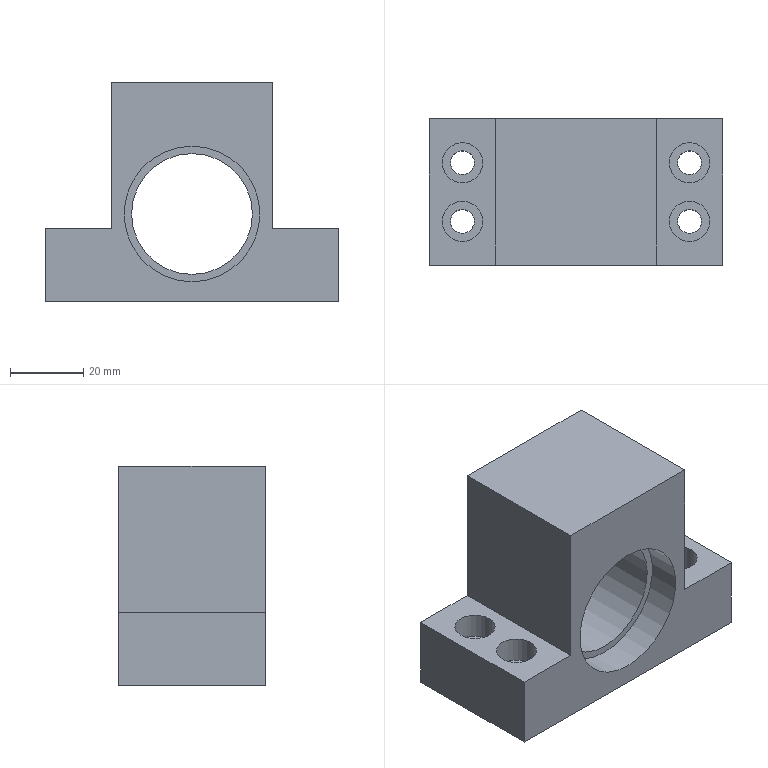Part | NX | features CBORE_HOLE 5, DATUM_CSYS 5, SKETCH 4, EXTRUDE 2, HOLE PACKAGE 2 | 1 solid | 25 faces | box 80 x 40 x 60 mm | volume 93822 mm3 | plane 15 | cylinder 10 | commonest cylinder face diameters 6.5 x4 11 x4 33 x1 37 x1
STEP:
#1=CARTESIAN_POINT('',(22.,20.,30.));
#2=VERTEX_POINT('',#1);
#3=CARTESIAN_POINT('',(22.,-20.,30.));
#4=VERTEX_POINT('',#3);
#5=CARTESIAN_POINT('',(22.,24.,30.));
#6=DIRECTION('',(0.,-1.,0.));
#7=VECTOR('',#6,1000.);
#8=LINE('',#5,#7);
#9=EDGE_CURVE('',#2,#4,#8,.T.);
#10=ORIENTED_EDGE('',*,*,#9,.F.);
#11=CARTESIAN_POINT('',(-22.,20.,30.));
#12=VERTEX_POINT('',#11);
#13=CARTESIAN_POINT('',(40.,20.,30.));
#14=DIRECTION('',(-1.,0.,0.));
#15=VECTOR('',#14,1000.);
#16=LINE('',#13,#15);
#17=EDGE_CURVE('',#2,#12,#16,.T.);
#18=ORIENTED_EDGE('',*,*,#17,.T.);
#19=CARTESIAN_POINT('',(-22.,-20.,30.));
#20=VERTEX_POINT('',#19);
#21=CARTESIAN_POINT('',(-22.,24.,30.));
#22=DIRECTION('',(0.,-1.,0.));
#23=VECTOR('',#22,1000.);
#24=LINE('',#21,#23);
#25=EDGE_CURVE('',#12,#20,#24,.T.);
#26=ORIENTED_EDGE('',*,*,#25,.T.);
#27=CARTESIAN_POINT('',(40.,-20.,30.));
#28=DIRECTION('',(-1.,0.,0.));
#29=VECTOR('',#28,1000.);
#30=LINE('',#27,#29);
#31=EDGE_CURVE('',#4,#20,#30,.T.);
#32=ORIENTED_EDGE('',*,*,#31,.F.);
#33=EDGE_LOOP('',(#10,#18,#26,#32));
#34=FACE_BOUND('',#33,.T.);
#35=CARTESIAN_POINT('',(40.,-20.,30.));
#36=DIRECTION('',(0.,0.,-1.));
#37=DIRECTION('',(-1.,0.,0.));
#38=AXIS2_PLACEMENT_3D('',#35,#36,#37);
#39=PLANE('',#38);
#40=ADVANCED_FACE('',(#34),#39,.F.);
#41=CARTESIAN_POINT('',(-40.,20.,-10.));
#42=VERTEX_POINT('',#41);
#43=CARTESIAN_POINT('',(-40.,-20.,-10.));
#44=VERTEX_POINT('',#43);
#45=CARTESIAN_POINT('',(-40.,24.,-10.));
#46=DIRECTION('',(0.,-1.,0.));
#47=VECTOR('',#46,1000.);
#48=LINE('',#45,#47);
#49=EDGE_CURVE('',#42,#44,#48,.T.);
#50=ORIENTED_EDGE('',*,*,#49,.F.);
#51=CARTESIAN_POINT('',(-40.,20.,-30.));
#52=VERTEX_POINT('',#51);
#53=CARTESIAN_POINT('',(-40.,20.,30.));
#54=DIRECTION('',(0.,0.,-1.));
#55=VECTOR('',#54,1000.);
#56=LINE('',#53,#55);
#57=EDGE_CURVE('',#42,#52,#56,.T.);
#58=ORIENTED_EDGE('',*,*,#57,.T.);
#59=CARTESIAN_POINT('',(-40.,-20.,-30.));
#60=VERTEX_POINT('',#59);
#61=CARTESIAN_POINT('',(-40.,-20.,-30.));
#62=DIRECTION('',(0.,1.,0.));
#63=VECTOR('',#62,1000.);
#64=LINE('',#61,#63);
#65=EDGE_CURVE('',#60,#52,#64,.T.);
#66=ORIENTED_EDGE('',*,*,#65,.F.);
#67=CARTESIAN_POINT('',(-40.,-20.,30.));
#68=DIRECTION('',(0.,0.,-1.));
#69=VECTOR('',#68,1000.);
#70=LINE('',#67,#69);
#71=EDGE_CURVE('',#44,#60,#70,.T.);
#72=ORIENTED_EDGE('',*,*,#71,.F.);
#73=EDGE_LOOP('',(#50,#58,#66,#72));
#74=FACE_BOUND('',#73,.T.);
#75=CARTESIAN_POINT('',(-40.,-20.,30.));
#76=DIRECTION('',(1.,0.,0.));
#77=DIRECTION('',(0.,0.,-1.));
#78=AXIS2_PLACEMENT_3D('',#75,#76,#77);
#79=PLANE('',#78);
#80=ADVANCED_FACE('',(#74),#79,.F.);
#81=CARTESIAN_POINT('',(34.25,8.,-30.));
#82=VERTEX_POINT('',#81);
#83=CARTESIAN_POINT('',(31.,8.,-30.));
#84=DIRECTION('',(0.,0.,1.));
#85=DIRECTION('',(1.,0.,0.));
#86=AXIS2_PLACEMENT_3D('',#83,#84,#85);
#87=CIRCLE('',#86,3.25);
#88=EDGE_CURVE('',#82,#82,#87,.T.);
#89=ORIENTED_EDGE('',*,*,#88,.T.);
#90=EDGE_LOOP('',(#89));
#91=FACE_BOUND('',#90,.T.);
#92=CARTESIAN_POINT('',(34.25,-8.,-30.));
#93=VERTEX_POINT('',#92);
#94=CARTESIAN_POINT('',(31.,-8.,-30.));
#95=DIRECTION('',(0.,0.,1.));
#96=DIRECTION('',(1.,0.,0.));
#97=AXIS2_PLACEMENT_3D('',#94,#95,#96);
#98=CIRCLE('',#97,3.25);
#99=EDGE_CURVE('',#93,#93,#98,.T.);
#100=ORIENTED_EDGE('',*,*,#99,.T.);
#101=EDGE_LOOP('',(#100));
#102=FACE_BOUND('',#101,.T.);
#103=CARTESIAN_POINT('',(-27.75,8.,-30.));
#104=VERTEX_POINT('',#103);
#105=CARTESIAN_POINT('',(-31.,8.,-30.));
#106=DIRECTION('',(0.,0.,1.));
#107=DIRECTION('',(1.,0.,0.));
#108=AXIS2_PLACEMENT_3D('',#105,#106,#107);
#109=CIRCLE('',#108,3.25);
#110=EDGE_CURVE('',#104,#104,#109,.T.);
#111=ORIENTED_EDGE('',*,*,#110,.T.);
#112=EDGE_LOOP('',(#111));
#113=FACE_BOUND('',#112,.T.);
#114=CARTESIAN_POINT('',(-27.75,-8.,-30.));
#115=VERTEX_POINT('',#114);
#116=CARTESIAN_POINT('',(-31.,-8.,-30.));
#117=DIRECTION('',(0.,0.,1.));
#118=DIRECTION('',(1.,0.,0.));
#119=AXIS2_PLACEMENT_3D('',#116,#117,#118);
#120=CIRCLE('',#119,3.25);
#121=EDGE_CURVE('',#115,#115,#120,.T.);
#122=ORIENTED_EDGE('',*,*,#121,.T.);
#123=EDGE_LOOP('',(#122));
#124=FACE_BOUND('',#123,.T.);
#125=CARTESIAN_POINT('',(40.,20.,-30.));
#126=VERTEX_POINT('',#125);
#127=CARTESIAN_POINT('',(-40.,20.,-30.));
#128=DIRECTION('',(1.,0.,0.));
#129=VECTOR('',#128,1000.);
#130=LINE('',#127,#129);
#131=EDGE_CURVE('',#52,#126,#130,.T.);
#132=ORIENTED_EDGE('',*,*,#131,.T.);
#133=CARTESIAN_POINT('',(40.,-20.,-30.));
#134=VERTEX_POINT('',#133);
#135=CARTESIAN_POINT('',(40.,-20.,-30.));
#136=DIRECTION('',(0.,1.,0.));
#137=VECTOR('',#136,1000.);
#138=LINE('',#135,#137);
#139=EDGE_CURVE('',#134,#126,#138,.T.);
#140=ORIENTED_EDGE('',*,*,#139,.F.);
#141=CARTESIAN_POINT('',(-40.,-20.,-30.));
#142=DIRECTION('',(1.,0.,0.));
#143=VECTOR('',#142,1000.);
#144=LINE('',#141,#143);
#145=EDGE_CURVE('',#60,#134,#144,.T.);
#146=ORIENTED_EDGE('',*,*,#145,.F.);
#147=ORIENTED_EDGE('',*,*,#65,.T.);
#148=EDGE_LOOP('',(#132,#140,#146,#147));
#149=FACE_BOUND('',#148,.T.);
#150=CARTESIAN_POINT('',(-40.,-20.,-30.));
#151=DIRECTION('',(0.,0.,1.));
#152=DIRECTION('',(1.,0.,0.));
#153=AXIS2_PLACEMENT_3D('',#150,#151,#152);
#154=PLANE('',#153);
#155=ADVANCED_FACE('',(#91,#102,#113,#124,#149),#154,.F.);
#156=CARTESIAN_POINT('',(40.,20.,-10.));
#157=VERTEX_POINT('',#156);
#158=CARTESIAN_POINT('',(40.,20.,-30.));
#159=DIRECTION('',(0.,0.,1.));
#160=VECTOR('',#159,1000.);
#161=LINE('',#158,#160);
#162=EDGE_CURVE('',#126,#157,#161,.T.);
#163=ORIENTED_EDGE('',*,*,#162,.T.);
#164=CARTESIAN_POINT('',(40.,-20.,-10.));
#165=VERTEX_POINT('',#164);
#166=CARTESIAN_POINT('',(40.,24.,-10.));
#167=DIRECTION('',(0.,-1.,0.));
#168=VECTOR('',#167,1000.);
#169=LINE('',#166,#168);
#170=EDGE_CURVE('',#157,#165,#169,.T.);
#171=ORIENTED_EDGE('',*,*,#170,.T.);
#172=CARTESIAN_POINT('',(40.,-20.,-30.));
#173=DIRECTION('',(0.,0.,1.));
#174=VECTOR('',#173,1000.);
#175=LINE('',#172,#174);
#176=EDGE_CURVE('',#134,#165,#175,.T.);
#177=ORIENTED_EDGE('',*,*,#176,.F.);
#178=ORIENTED_EDGE('',*,*,#139,.T.);
#179=EDGE_LOOP('',(#163,#171,#177,#178));
#180=FACE_BOUND('',#179,.T.);
#181=CARTESIAN_POINT('',(40.,-20.,-30.));
#182=DIRECTION('',(-1.,0.,0.));
#183=DIRECTION('',(0.,0.,1.));
#184=AXIS2_PLACEMENT_3D('',#181,#182,#183);
#185=PLANE('',#184);
#186=ADVANCED_FACE('',(#180),#185,.F.);
#187=CARTESIAN_POINT('',(22.,-20.,-10.));
#188=VERTEX_POINT('',#187);
#189=CARTESIAN_POINT('',(22.,-20.,30.));
#190=DIRECTION('',(0.,0.,-1.));
#191=VECTOR('',#190,1000.);
#192=LINE('',#189,#191);
#193=EDGE_CURVE('',#4,#188,#192,.T.);
#194=ORIENTED_EDGE('',*,*,#193,.F.);
#195=ORIENTED_EDGE('',*,*,#31,.T.);
#196=CARTESIAN_POINT('',(-22.,-20.,-10.));
#197=VERTEX_POINT('',#196);
#198=CARTESIAN_POINT('',(-22.,-20.,-10.));
#199=DIRECTION('',(0.,0.,1.));
#200=VECTOR('',#199,1000.);
#201=LINE('',#198,#200);
#202=EDGE_CURVE('',#197,#20,#201,.T.);
#203=ORIENTED_EDGE('',*,*,#202,.F.);
#204=CARTESIAN_POINT('',(-40.,-20.,-10.));
#205=DIRECTION('',(1.,0.,0.));
#206=VECTOR('',#205,1000.);
#207=LINE('',#204,#206);
#208=EDGE_CURVE('',#44,#197,#207,.T.);
#209=ORIENTED_EDGE('',*,*,#208,.F.);
#210=ORIENTED_EDGE('',*,*,#71,.T.);
#211=ORIENTED_EDGE('',*,*,#145,.T.);
#212=ORIENTED_EDGE('',*,*,#176,.T.);
#213=CARTESIAN_POINT('',(22.,-20.,-10.));
#214=DIRECTION('',(1.,0.,0.));
#215=VECTOR('',#214,1000.);
#216=LINE('',#213,#215);
#217=EDGE_CURVE('',#188,#165,#216,.T.);
#218=ORIENTED_EDGE('',*,*,#217,.F.);
#219=EDGE_LOOP('',(#194,#195,#203,#209,#210,#211,#212,#218));
#220=FACE_BOUND('',#219,.T.);
#221=CARTESIAN_POINT('',(0.,-20.,12.5));
#222=VERTEX_POINT('',#221);
#223=CARTESIAN_POINT('',(0.,-20.,-6.));
#224=DIRECTION('',(0.,1.,0.));
#225=DIRECTION('',(0.,0.,1.));
#226=AXIS2_PLACEMENT_3D('',#223,#224,#225);
#227=CIRCLE('',#226,18.5);
#228=EDGE_CURVE('',#222,#222,#227,.T.);
#229=ORIENTED_EDGE('',*,*,#228,.T.);
#230=EDGE_LOOP('',(#229));
#231=FACE_BOUND('',#230,.T.);
#232=CARTESIAN_POINT('',(0.,-20.,0.));
#233=DIRECTION('',(0.,-1.,0.));
#234=DIRECTION('',(0.,0.,-1.));
#235=AXIS2_PLACEMENT_3D('',#232,#233,#234);
#236=PLANE('',#235);
#237=ADVANCED_FACE('',(#220,#231),#236,.T.);
#238=CARTESIAN_POINT('',(0.,20.,-22.5));
#239=VERTEX_POINT('',#238);
#240=CARTESIAN_POINT('',(0.,20.,-6.));
#241=DIRECTION('',(0.,-1.,0.));
#242=DIRECTION('',(0.,0.,-1.));
#243=AXIS2_PLACEMENT_3D('',#240,#241,#242);
#244=CIRCLE('',#243,16.5);
#245=EDGE_CURVE('',#239,#239,#244,.T.);
#246=ORIENTED_EDGE('',*,*,#245,.T.);
#247=EDGE_LOOP('',(#246));
#248=FACE_BOUND('',#247,.T.);
#249=ORIENTED_EDGE('',*,*,#17,.F.);
#250=CARTESIAN_POINT('',(22.,20.,-10.));
#251=VERTEX_POINT('',#250);
#252=CARTESIAN_POINT('',(22.,20.,0.));
#253=DIRECTION('',(0.,0.,-1.));
#254=VECTOR('',#253,1000.);
#255=LINE('',#252,#254);
#256=EDGE_CURVE('',#2,#251,#255,.T.);
#257=ORIENTED_EDGE('',*,*,#256,.T.);
#258=CARTESIAN_POINT('',(0.,20.,-10.));
#259=DIRECTION('',(1.,0.,0.));
#260=VECTOR('',#259,1000.);
#261=LINE('',#258,#260);
#262=EDGE_CURVE('',#251,#157,#261,.T.);
#263=ORIENTED_EDGE('',*,*,#262,.T.);
#264=ORIENTED_EDGE('',*,*,#162,.F.);
#265=ORIENTED_EDGE('',*,*,#131,.F.);
#266=ORIENTED_EDGE('',*,*,#57,.F.);
#267=CARTESIAN_POINT('',(-22.,20.,-10.));
#268=VERTEX_POINT('',#267);
#269=CARTESIAN_POINT('',(0.,20.,-10.));
#270=DIRECTION('',(1.,0.,0.));
#271=VECTOR('',#270,1000.);
#272=LINE('',#269,#271);
#273=EDGE_CURVE('',#42,#268,#272,.T.);
#274=ORIENTED_EDGE('',*,*,#273,.T.);
#275=CARTESIAN_POINT('',(-22.,20.,0.));
#276=DIRECTION('',(0.,0.,1.));
#277=VECTOR('',#276,1000.);
#278=LINE('',#275,#277);
#279=EDGE_CURVE('',#268,#12,#278,.T.);
#280=ORIENTED_EDGE('',*,*,#279,.T.);
#281=EDGE_LOOP('',(#249,#257,#263,#264,#265,#266,#274,#280));
#282=FACE_BOUND('',#281,.T.);
#283=CARTESIAN_POINT('',(0.,20.,0.));
#284=DIRECTION('',(0.,-1.,0.));
#285=DIRECTION('',(0.,0.,-1.));
#286=AXIS2_PLACEMENT_3D('',#283,#284,#285);
#287=PLANE('',#286);
#288=ADVANCED_FACE('',(#248,#282),#287,.F.);
#289=CARTESIAN_POINT('',(0.,-11.,10.5));
#290=VERTEX_POINT('',#289);
#291=CARTESIAN_POINT('',(0.,-11.,-6.));
#292=DIRECTION('',(0.,1.,0.));
#293=DIRECTION('',(0.,0.,1.));
#294=AXIS2_PLACEMENT_3D('',#291,#292,#293);
#295=CIRCLE('',#294,16.5);
#296=EDGE_CURVE('',#290,#290,#295,.F.);
#297=ORIENTED_EDGE('',*,*,#296,.T.);
#298=EDGE_LOOP('',(#297));
#299=FACE_BOUND('',#298,.T.);
#300=ORIENTED_EDGE('',*,*,#245,.F.);
#301=EDGE_LOOP('',(#300));
#302=FACE_BOUND('',#301,.T.);
#303=CARTESIAN_POINT('',(0.,58.932,-6.));
#304=DIRECTION('',(0.,1.,0.));
#305=DIRECTION('',(0.,0.,1.));
#306=AXIS2_PLACEMENT_3D('',#303,#304,#305);
#307=CYLINDRICAL_SURFACE('',#306,16.5);
#308=ADVANCED_FACE('',(#299,#302),#307,.F.);
#309=ORIENTED_EDGE('',*,*,#296,.F.);
#310=EDGE_LOOP('',(#309));
#311=FACE_BOUND('',#310,.T.);
#312=CARTESIAN_POINT('',(0.,-11.,12.5));
#313=VERTEX_POINT('',#312);
#314=CARTESIAN_POINT('',(0.,-11.,-6.));
#315=DIRECTION('',(0.,1.,0.));
#316=DIRECTION('',(0.,0.,1.));
#317=AXIS2_PLACEMENT_3D('',#314,#315,#316);
#318=CIRCLE('',#317,18.5);
#319=EDGE_CURVE('',#313,#313,#318,.F.);
#320=ORIENTED_EDGE('',*,*,#319,.T.);
#321=EDGE_LOOP('',(#320));
#322=FACE_BOUND('',#321,.T.);
#323=CARTESIAN_POINT('',(0.,-11.,-6.));
#324=DIRECTION('',(0.,1.,0.));
#325=DIRECTION('',(0.,0.,1.));
#326=AXIS2_PLACEMENT_3D('',#323,#324,#325);
#327=PLANE('',#326);
#328=ADVANCED_FACE('',(#311,#322),#327,.F.);
#329=ORIENTED_EDGE('',*,*,#319,.F.);
#330=EDGE_LOOP('',(#329));
#331=FACE_BOUND('',#330,.T.);
#332=ORIENTED_EDGE('',*,*,#228,.F.);
#333=EDGE_LOOP('',(#332));
#334=FACE_BOUND('',#333,.T.);
#335=CARTESIAN_POINT('',(0.,-20.,-6.));
#336=DIRECTION('',(0.,1.,0.));
#337=DIRECTION('',(0.,0.,1.));
#338=AXIS2_PLACEMENT_3D('',#335,#336,#337);
#339=CYLINDRICAL_SURFACE('',#338,18.5);
#340=ADVANCED_FACE('',(#331,#334),#339,.F.);
#341=CARTESIAN_POINT('',(-36.5,8.,-10.));
#342=VERTEX_POINT('',#341);
#343=CARTESIAN_POINT('',(-31.,8.,-10.));
#344=DIRECTION('',(0.,0.,-1.));
#345=DIRECTION('',(-1.,0.,0.));
#346=AXIS2_PLACEMENT_3D('',#343,#344,#345);
#347=CIRCLE('',#346,5.5);
#348=EDGE_CURVE('',#342,#342,#347,.T.);
#349=ORIENTED_EDGE('',*,*,#348,.T.);
#350=EDGE_LOOP('',(#349));
#351=FACE_BOUND('',#350,.T.);
#352=CARTESIAN_POINT('',(-36.5,-8.,-10.));
#353=VERTEX_POINT('',#352);
#354=CARTESIAN_POINT('',(-31.,-8.,-10.));
#355=DIRECTION('',(0.,0.,-1.));
#356=DIRECTION('',(-1.,0.,0.));
#357=AXIS2_PLACEMENT_3D('',#354,#355,#356);
#358=CIRCLE('',#357,5.5);
#359=EDGE_CURVE('',#353,#353,#358,.T.);
#360=ORIENTED_EDGE('',*,*,#359,.T.);
#361=EDGE_LOOP('',(#360));
#362=FACE_BOUND('',#361,.T.);
#363=ORIENTED_EDGE('',*,*,#49,.T.);
#364=ORIENTED_EDGE('',*,*,#208,.T.);
#365=CARTESIAN_POINT('',(-22.,24.,-10.));
#366=DIRECTION('',(0.,-1.,0.));
#367=VECTOR('',#366,1000.);
#368=LINE('',#365,#367);
#369=EDGE_CURVE('',#197,#268,#368,.F.);
#370=ORIENTED_EDGE('',*,*,#369,.T.);
#371=ORIENTED_EDGE('',*,*,#273,.F.);
#372=EDGE_LOOP('',(#363,#364,#370,#371));
#373=FACE_BOUND('',#372,.T.);
#374=CARTESIAN_POINT('',(-40.,24.,-10.));
#375=DIRECTION('',(0.,0.,-1.));
#376=DIRECTION('',(-1.,0.,0.));
#377=AXIS2_PLACEMENT_3D('',#374,#375,#376);
#378=PLANE('',#377);
#379=ADVANCED_FACE('',(#351,#362,#373),#378,.F.);
#380=ORIENTED_EDGE('',*,*,#369,.F.);
#381=ORIENTED_EDGE('',*,*,#202,.T.);
#382=ORIENTED_EDGE('',*,*,#25,.F.);
#383=ORIENTED_EDGE('',*,*,#279,.F.);
#384=EDGE_LOOP('',(#380,#381,#382,#383));
#385=FACE_BOUND('',#384,.T.);
#386=CARTESIAN_POINT('',(-22.,24.,-10.));
#387=DIRECTION('',(1.,0.,0.));
#388=DIRECTION('',(0.,0.,-1.));
#389=AXIS2_PLACEMENT_3D('',#386,#387,#388);
#390=PLANE('',#389);
#391=ADVANCED_FACE('',(#385),#390,.F.);
#392=ORIENTED_EDGE('',*,*,#9,.T.);
#393=ORIENTED_EDGE('',*,*,#193,.T.);
#394=CARTESIAN_POINT('',(22.,24.,-10.));
#395=DIRECTION('',(0.,-1.,0.));
#396=VECTOR('',#395,1000.);
#397=LINE('',#394,#396);
#398=EDGE_CURVE('',#188,#251,#397,.F.);
#399=ORIENTED_EDGE('',*,*,#398,.T.);
#400=ORIENTED_EDGE('',*,*,#256,.F.);
#401=EDGE_LOOP('',(#392,#393,#399,#400));
#402=FACE_BOUND('',#401,.T.);
#403=CARTESIAN_POINT('',(22.,24.,30.));
#404=DIRECTION('',(-1.,0.,0.));
#405=DIRECTION('',(0.,0.,1.));
#406=AXIS2_PLACEMENT_3D('',#403,#404,#405);
#407=PLANE('',#406);
#408=ADVANCED_FACE('',(#402),#407,.F.);
#409=CARTESIAN_POINT('',(25.5,8.,-10.));
#410=VERTEX_POINT('',#409);
#411=CARTESIAN_POINT('',(31.,8.,-10.));
#412=DIRECTION('',(0.,0.,-1.));
#413=DIRECTION('',(-1.,0.,0.));
#414=AXIS2_PLACEMENT_3D('',#411,#412,#413);
#415=CIRCLE('',#414,5.5);
#416=EDGE_CURVE('',#410,#410,#415,.T.);
#417=ORIENTED_EDGE('',*,*,#416,.T.);
#418=EDGE_LOOP('',(#417));
#419=FACE_BOUND('',#418,.T.);
#420=CARTESIAN_POINT('',(25.5,-8.,-10.));
#421=VERTEX_POINT('',#420);
#422=CARTESIAN_POINT('',(31.,-8.,-10.));
#423=DIRECTION('',(0.,0.,-1.));
#424=DIRECTION('',(-1.,0.,0.));
#425=AXIS2_PLACEMENT_3D('',#422,#423,#424);
#426=CIRCLE('',#425,5.5);
#427=EDGE_CURVE('',#421,#421,#426,.T.);
#428=ORIENTED_EDGE('',*,*,#427,.T.);
#429=EDGE_LOOP('',(#428));
#430=FACE_BOUND('',#429,.T.);
#431=ORIENTED_EDGE('',*,*,#398,.F.);
#432=ORIENTED_EDGE('',*,*,#217,.T.);
#433=ORIENTED_EDGE('',*,*,#170,.F.);
#434=ORIENTED_EDGE('',*,*,#262,.F.);
#435=EDGE_LOOP('',(#431,#432,#433,#434));
#436=FACE_BOUND('',#435,.T.);
#437=CARTESIAN_POINT('',(22.,24.,-10.));
#438=DIRECTION('',(0.,0.,-1.));
#439=DIRECTION('',(-1.,0.,0.));
#440=AXIS2_PLACEMENT_3D('',#437,#438,#439);
#441=PLANE('',#440);
#442=ADVANCED_FACE('',(#419,#430,#436),#441,.F.);
#443=CARTESIAN_POINT('',(-34.25,-8.,-17.));
#444=VERTEX_POINT('',#443);
#445=CARTESIAN_POINT('',(-31.,-8.,-17.));
#446=DIRECTION('',(0.,0.,-1.));
#447=DIRECTION('',(-1.,0.,0.));
#448=AXIS2_PLACEMENT_3D('',#445,#446,#447);
#449=CIRCLE('',#448,3.25);
#450=EDGE_CURVE('',#444,#444,#449,.F.);
#451=ORIENTED_EDGE('',*,*,#450,.T.);
#452=EDGE_LOOP('',(#451));
#453=FACE_BOUND('',#452,.T.);
#454=ORIENTED_EDGE('',*,*,#121,.F.);
#455=EDGE_LOOP('',(#454));
#456=FACE_BOUND('',#455,.T.);
#457=CARTESIAN_POINT('',(-31.,-8.,-49.84));
#458=DIRECTION('',(0.,0.,-1.));
#459=DIRECTION('',(-1.,0.,0.));
#460=AXIS2_PLACEMENT_3D('',#457,#458,#459);
#461=CYLINDRICAL_SURFACE('',#460,3.25);
#462=ADVANCED_FACE('',(#453,#456),#461,.F.);
#463=ORIENTED_EDGE('',*,*,#450,.F.);
#464=EDGE_LOOP('',(#463));
#465=FACE_BOUND('',#464,.T.);
#466=CARTESIAN_POINT('',(-36.5,-8.,-17.));
#467=VERTEX_POINT('',#466);
#468=CARTESIAN_POINT('',(-31.,-8.,-17.));
#469=DIRECTION('',(0.,0.,-1.));
#470=DIRECTION('',(-1.,0.,0.));
#471=AXIS2_PLACEMENT_3D('',#468,#469,#470);
#472=CIRCLE('',#471,5.5);
#473=EDGE_CURVE('',#467,#467,#472,.F.);
#474=ORIENTED_EDGE('',*,*,#473,.T.);
#475=EDGE_LOOP('',(#474));
#476=FACE_BOUND('',#475,.T.);
#477=CARTESIAN_POINT('',(-31.,-8.,-17.));
#478=DIRECTION('',(0.,0.,-1.));
#479=DIRECTION('',(-1.,0.,0.));
#480=AXIS2_PLACEMENT_3D('',#477,#478,#479);
#481=PLANE('',#480);
#482=ADVANCED_FACE('',(#465,#476),#481,.F.);
#483=ORIENTED_EDGE('',*,*,#473,.F.);
#484=EDGE_LOOP('',(#483));
#485=FACE_BOUND('',#484,.T.);
#486=ORIENTED_EDGE('',*,*,#359,.F.);
#487=EDGE_LOOP('',(#486));
#488=FACE_BOUND('',#487,.T.);
#489=CARTESIAN_POINT('',(-31.,-8.,-10.));
#490=DIRECTION('',(0.,0.,-1.));
#491=DIRECTION('',(-1.,0.,0.));
#492=AXIS2_PLACEMENT_3D('',#489,#490,#491);
#493=CYLINDRICAL_SURFACE('',#492,5.5);
#494=ADVANCED_FACE('',(#485,#488),#493,.F.);
#495=CARTESIAN_POINT('',(-34.25,8.,-17.));
#496=VERTEX_POINT('',#495);
#497=CARTESIAN_POINT('',(-31.,8.,-17.));
#498=DIRECTION('',(0.,0.,-1.));
#499=DIRECTION('',(-1.,0.,0.));
#500=AXIS2_PLACEMENT_3D('',#497,#498,#499);
#501=CIRCLE('',#500,3.25);
#502=EDGE_CURVE('',#496,#496,#501,.F.);
#503=ORIENTED_EDGE('',*,*,#502,.T.);
#504=EDGE_LOOP('',(#503));
#505=FACE_BOUND('',#504,.T.);
#506=ORIENTED_EDGE('',*,*,#110,.F.);
#507=EDGE_LOOP('',(#506));
#508=FACE_BOUND('',#507,.T.);
#509=CARTESIAN_POINT('',(-31.,8.,-49.84));
#510=DIRECTION('',(0.,0.,-1.));
#511=DIRECTION('',(-1.,0.,0.));
#512=AXIS2_PLACEMENT_3D('',#509,#510,#511);
#513=CYLINDRICAL_SURFACE('',#512,3.25);
#514=ADVANCED_FACE('',(#505,#508),#513,.F.);
#515=ORIENTED_EDGE('',*,*,#502,.F.);
#516=EDGE_LOOP('',(#515));
#517=FACE_BOUND('',#516,.T.);
#518=CARTESIAN_POINT('',(-36.5,8.,-17.));
#519=VERTEX_POINT('',#518);
#520=CARTESIAN_POINT('',(-31.,8.,-17.));
#521=DIRECTION('',(0.,0.,-1.));
#522=DIRECTION('',(-1.,0.,0.));
#523=AXIS2_PLACEMENT_3D('',#520,#521,#522);
#524=CIRCLE('',#523,5.5);
#525=EDGE_CURVE('',#519,#519,#524,.F.);
#526=ORIENTED_EDGE('',*,*,#525,.T.);
#527=EDGE_LOOP('',(#526));
#528=FACE_BOUND('',#527,.T.);
#529=CARTESIAN_POINT('',(-31.,8.,-17.));
#530=DIRECTION('',(0.,0.,-1.));
#531=DIRECTION('',(-1.,0.,0.));
#532=AXIS2_PLACEMENT_3D('',#529,#530,#531);
#533=PLANE('',#532);
#534=ADVANCED_FACE('',(#517,#528),#533,.F.);
#535=ORIENTED_EDGE('',*,*,#525,.F.);
#536=EDGE_LOOP('',(#535));
#537=FACE_BOUND('',#536,.T.);
#538=ORIENTED_EDGE('',*,*,#348,.F.);
#539=EDGE_LOOP('',(#538));
#540=FACE_BOUND('',#539,.T.);
#541=CARTESIAN_POINT('',(-31.,8.,-10.));
#542=DIRECTION('',(0.,0.,-1.));
#543=DIRECTION('',(-1.,0.,0.));
#544=AXIS2_PLACEMENT_3D('',#541,#542,#543);
#545=CYLINDRICAL_SURFACE('',#544,5.5);
#546=ADVANCED_FACE('',(#537,#540),#545,.F.);
#547=CARTESIAN_POINT('',(27.75,-8.,-17.));
#548=VERTEX_POINT('',#547);
#549=CARTESIAN_POINT('',(31.,-8.,-17.));
#550=DIRECTION('',(0.,0.,-1.));
#551=DIRECTION('',(-1.,0.,0.));
#552=AXIS2_PLACEMENT_3D('',#549,#550,#551);
#553=CIRCLE('',#552,3.25);
#554=EDGE_CURVE('',#548,#548,#553,.F.);
#555=ORIENTED_EDGE('',*,*,#554,.T.);
#556=EDGE_LOOP('',(#555));
#557=FACE_BOUND('',#556,.T.);
#558=ORIENTED_EDGE('',*,*,#99,.F.);
#559=EDGE_LOOP('',(#558));
#560=FACE_BOUND('',#559,.T.);
#561=CARTESIAN_POINT('',(31.,-8.,-49.84));
#562=DIRECTION('',(0.,0.,-1.));
#563=DIRECTION('',(-1.,0.,0.));
#564=AXIS2_PLACEMENT_3D('',#561,#562,#563);
#565=CYLINDRICAL_SURFACE('',#564,3.25);
#566=ADVANCED_FACE('',(#557,#560),#565,.F.);
#567=ORIENTED_EDGE('',*,*,#554,.F.);
#568=EDGE_LOOP('',(#567));
#569=FACE_BOUND('',#568,.T.);
#570=CARTESIAN_POINT('',(25.5,-8.,-17.));
#571=VERTEX_POINT('',#570);
#572=CARTESIAN_POINT('',(31.,-8.,-17.));
#573=DIRECTION('',(0.,0.,-1.));
#574=DIRECTION('',(-1.,0.,0.));
#575=AXIS2_PLACEMENT_3D('',#572,#573,#574);
#576=CIRCLE('',#575,5.5);
#577=EDGE_CURVE('',#571,#571,#576,.F.);
#578=ORIENTED_EDGE('',*,*,#577,.T.);
#579=EDGE_LOOP('',(#578));
#580=FACE_BOUND('',#579,.T.);
#581=CARTESIAN_POINT('',(31.,-8.,-17.));
#582=DIRECTION('',(0.,0.,-1.));
#583=DIRECTION('',(-1.,0.,0.));
#584=AXIS2_PLACEMENT_3D('',#581,#582,#583);
#585=PLANE('',#584);
#586=ADVANCED_FACE('',(#569,#580),#585,.F.);
#587=ORIENTED_EDGE('',*,*,#577,.F.);
#588=EDGE_LOOP('',(#587));
#589=FACE_BOUND('',#588,.T.);
#590=ORIENTED_EDGE('',*,*,#427,.F.);
#591=EDGE_LOOP('',(#590));
#592=FACE_BOUND('',#591,.T.);
#593=CARTESIAN_POINT('',(31.,-8.,-10.));
#594=DIRECTION('',(0.,0.,-1.));
#595=DIRECTION('',(-1.,0.,0.));
#596=AXIS2_PLACEMENT_3D('',#593,#594,#595);
#597=CYLINDRICAL_SURFACE('',#596,5.5);
#598=ADVANCED_FACE('',(#589,#592),#597,.F.);
#599=CARTESIAN_POINT('',(27.75,8.,-17.));
#600=VERTEX_POINT('',#599);
#601=CARTESIAN_POINT('',(31.,8.,-17.));
#602=DIRECTION('',(0.,0.,-1.));
#603=DIRECTION('',(-1.,0.,0.));
#604=AXIS2_PLACEMENT_3D('',#601,#602,#603);
#605=CIRCLE('',#604,3.25);
#606=EDGE_CURVE('',#600,#600,#605,.F.);
#607=ORIENTED_EDGE('',*,*,#606,.T.);
#608=EDGE_LOOP('',(#607));
#609=FACE_BOUND('',#608,.T.);
#610=ORIENTED_EDGE('',*,*,#88,.F.);
#611=EDGE_LOOP('',(#610));
#612=FACE_BOUND('',#611,.T.);
#613=CARTESIAN_POINT('',(31.,8.,-49.84));
#614=DIRECTION('',(0.,0.,-1.));
#615=DIRECTION('',(-1.,0.,0.));
#616=AXIS2_PLACEMENT_3D('',#613,#614,#615);
#617=CYLINDRICAL_SURFACE('',#616,3.25);
#618=ADVANCED_FACE('',(#609,#612),#617,.F.);
#619=ORIENTED_EDGE('',*,*,#606,.F.);
#620=EDGE_LOOP('',(#619));
#621=FACE_BOUND('',#620,.T.);
#622=CARTESIAN_POINT('',(25.5,8.,-17.));
#623=VERTEX_POINT('',#622);
#624=CARTESIAN_POINT('',(31.,8.,-17.));
#625=DIRECTION('',(0.,0.,-1.));
#626=DIRECTION('',(-1.,0.,0.));
#627=AXIS2_PLACEMENT_3D('',#624,#625,#626);
#628=CIRCLE('',#627,5.5);
#629=EDGE_CURVE('',#623,#623,#628,.F.);
#630=ORIENTED_EDGE('',*,*,#629,.T.);
#631=EDGE_LOOP('',(#630));
#632=FACE_BOUND('',#631,.T.);
#633=CARTESIAN_POINT('',(31.,8.,-17.));
#634=DIRECTION('',(0.,0.,-1.));
#635=DIRECTION('',(-1.,0.,0.));
#636=AXIS2_PLACEMENT_3D('',#633,#634,#635);
#637=PLANE('',#636);
#638=ADVANCED_FACE('',(#621,#632),#637,.F.);
#639=ORIENTED_EDGE('',*,*,#629,.F.);
#640=EDGE_LOOP('',(#639));
#641=FACE_BOUND('',#640,.T.);
#642=ORIENTED_EDGE('',*,*,#416,.F.);
#643=EDGE_LOOP('',(#642));
#644=FACE_BOUND('',#643,.T.);
#645=CARTESIAN_POINT('',(31.,8.,-10.));
#646=DIRECTION('',(0.,0.,-1.));
#647=DIRECTION('',(-1.,0.,0.));
#648=AXIS2_PLACEMENT_3D('',#645,#646,#647);
#649=CYLINDRICAL_SURFACE('',#648,5.5);
#650=ADVANCED_FACE('',(#641,#644),#649,.F.);
#651=CLOSED_SHELL('',(#40,#80,#155,#186,#237,#288,#308,#328,#340,#379,#391,#408,#442,#462,#482,#494,#514,#534,#546,#566,#586,#598,#618,#638,#650));
#652=MANIFOLD_SOLID_BREP('',#651);
#653=(LENGTH_UNIT()NAMED_UNIT(*)SI_UNIT(.MILLI.,.METRE.));
#654=UNCERTAINTY_MEASURE_WITH_UNIT(LENGTH_MEASURE(0.00001),#653,'','');
#655=(NAMED_UNIT(*)PLANE_ANGLE_UNIT()SI_UNIT($,.RADIAN.));
#656=(NAMED_UNIT(*)SI_UNIT($,.STERADIAN.)SOLID_ANGLE_UNIT());
#657=(GEOMETRIC_REPRESENTATION_CONTEXT(3)GLOBAL_UNCERTAINTY_ASSIGNED_CONTEXT((#654))GLOBAL_UNIT_ASSIGNED_CONTEXT((#653,#655,#656))REPRESENTATION_CONTEXT('',''));
#658=ADVANCED_BREP_SHAPE_REPRESENTATION('',(#652),#657);